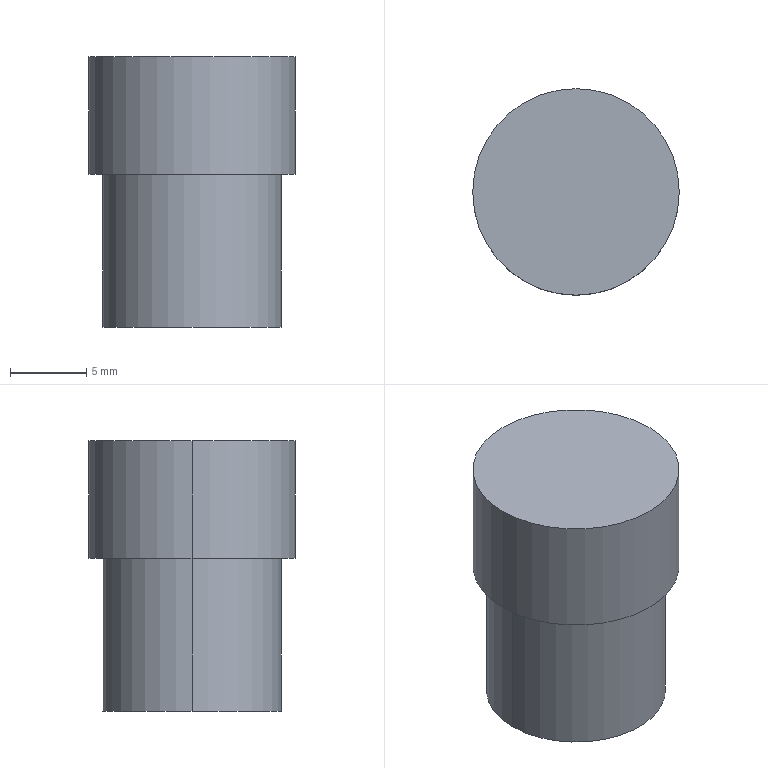Part | SolidWorks | features ICE 2, Extrusion 1 | 1 solid | 7 faces | box 13.5 x 13.5 x 17.7 mm | volume 2177 mm3 | cylinder 4 | plane 3 | commonest cylinder face diameters 11.7 x2 13.5 x2
STEP:
#1=CARTESIAN_POINT('',(44.682,-8.106,-13.2));
#2=VERTEX_POINT('',#1);
#3=CARTESIAN_POINT('',(56.382,-8.106,-13.2));
#4=VERTEX_POINT('',#3);
#5=CARTESIAN_POINT('',(50.532,-8.106,-13.2));
#6=DIRECTION('',(0.,0.,-1.));
#7=DIRECTION('',(-1.,0.,0.));
#8=AXIS2_PLACEMENT_3D('',#5,#6,#7);
#9=CIRCLE('',#8,5.85);
#10=EDGE_CURVE('',#2,#4,#9,.T.);
#11=ORIENTED_EDGE('',*,*,#10,.F.);
#12=CARTESIAN_POINT('',(44.682,-8.106,-3.2));
#13=VERTEX_POINT('',#12);
#14=CARTESIAN_POINT('',(44.682,-8.106,-13.2));
#15=DIRECTION('',(0.,0.,1.));
#16=VECTOR('',#15,1000.);
#17=LINE('',#14,#16);
#18=EDGE_CURVE('',#2,#13,#17,.T.);
#19=ORIENTED_EDGE('',*,*,#18,.T.);
#20=CARTESIAN_POINT('',(56.382,-8.106,-3.2));
#21=VERTEX_POINT('',#20);
#22=CARTESIAN_POINT('',(50.532,-8.106,-3.2));
#23=DIRECTION('',(0.,0.,-1.));
#24=DIRECTION('',(-1.,0.,0.));
#25=AXIS2_PLACEMENT_3D('',#22,#23,#24);
#26=CIRCLE('',#25,5.85);
#27=EDGE_CURVE('',#13,#21,#26,.T.);
#28=ORIENTED_EDGE('',*,*,#27,.T.);
#29=CARTESIAN_POINT('',(56.382,-8.106,-13.2));
#30=DIRECTION('',(0.,0.,1.));
#31=VECTOR('',#30,1000.);
#32=LINE('',#29,#31);
#33=EDGE_CURVE('',#4,#21,#32,.T.);
#34=ORIENTED_EDGE('',*,*,#33,.F.);
#35=EDGE_LOOP('',(#11,#19,#28,#34));
#36=FACE_OUTER_BOUND('',#35,.T.);
#37=CARTESIAN_POINT('',(50.532,-8.106,-13.2));
#38=DIRECTION('',(0.,0.,1.));
#39=DIRECTION('',(1.,0.,0.));
#40=AXIS2_PLACEMENT_3D('',#37,#38,#39);
#41=CYLINDRICAL_SURFACE('',#40,5.85);
#42=ADVANCED_FACE('',(#36),#41,.T.);
#43=CARTESIAN_POINT('',(57.282,-8.106,4.5));
#44=VERTEX_POINT('',#43);
#45=CARTESIAN_POINT('',(43.782,-8.106,4.5));
#46=VERTEX_POINT('',#45);
#47=CARTESIAN_POINT('',(50.532,-8.106,4.5));
#48=DIRECTION('',(0.,0.,1.));
#49=DIRECTION('',(1.,0.,0.));
#50=AXIS2_PLACEMENT_3D('',#47,#48,#49);
#51=CIRCLE('',#50,6.75);
#52=EDGE_CURVE('',#44,#46,#51,.T.);
#53=ORIENTED_EDGE('',*,*,#52,.F.);
#54=CARTESIAN_POINT('',(57.282,-8.106,-3.2));
#55=VERTEX_POINT('',#54);
#56=CARTESIAN_POINT('',(57.282,-8.106,4.5));
#57=DIRECTION('',(0.,0.,-1.));
#58=VECTOR('',#57,1000.);
#59=LINE('',#56,#58);
#60=EDGE_CURVE('',#44,#55,#59,.T.);
#61=ORIENTED_EDGE('',*,*,#60,.T.);
#62=CARTESIAN_POINT('',(43.782,-8.106,-3.2));
#63=VERTEX_POINT('',#62);
#64=CARTESIAN_POINT('',(50.532,-8.106,-3.2));
#65=DIRECTION('',(0.,0.,-1.));
#66=DIRECTION('',(-1.,0.,0.));
#67=AXIS2_PLACEMENT_3D('',#64,#65,#66);
#68=CIRCLE('',#67,6.75);
#69=EDGE_CURVE('',#63,#55,#68,.T.);
#70=ORIENTED_EDGE('',*,*,#69,.F.);
#71=CARTESIAN_POINT('',(43.782,-8.106,4.5));
#72=DIRECTION('',(0.,0.,-1.));
#73=VECTOR('',#72,1000.);
#74=LINE('',#71,#73);
#75=EDGE_CURVE('',#46,#63,#74,.T.);
#76=ORIENTED_EDGE('',*,*,#75,.F.);
#77=EDGE_LOOP('',(#53,#61,#70,#76));
#78=FACE_OUTER_BOUND('',#77,.T.);
#79=CARTESIAN_POINT('',(50.532,-8.106,4.5));
#80=DIRECTION('',(0.,0.,-1.));
#81=DIRECTION('',(-1.,0.,0.));
#82=AXIS2_PLACEMENT_3D('',#79,#80,#81);
#83=CYLINDRICAL_SURFACE('',#82,6.75);
#84=ADVANCED_FACE('',(#78),#83,.T.);
#85=ORIENTED_EDGE('',*,*,#60,.F.);
#86=CARTESIAN_POINT('',(50.532,-8.106,4.5));
#87=DIRECTION('',(0.,0.,1.));
#88=DIRECTION('',(1.,0.,0.));
#89=AXIS2_PLACEMENT_3D('',#86,#87,#88);
#90=CIRCLE('',#89,6.75);
#91=EDGE_CURVE('',#46,#44,#90,.T.);
#92=ORIENTED_EDGE('',*,*,#91,.F.);
#93=ORIENTED_EDGE('',*,*,#75,.T.);
#94=CARTESIAN_POINT('',(50.532,-8.106,-3.2));
#95=DIRECTION('',(0.,0.,-1.));
#96=DIRECTION('',(-1.,0.,0.));
#97=AXIS2_PLACEMENT_3D('',#94,#95,#96);
#98=CIRCLE('',#97,6.75);
#99=EDGE_CURVE('',#55,#63,#98,.T.);
#100=ORIENTED_EDGE('',*,*,#99,.F.);
#101=EDGE_LOOP('',(#85,#92,#93,#100));
#102=FACE_OUTER_BOUND('',#101,.T.);
#103=CARTESIAN_POINT('',(50.532,-8.106,4.5));
#104=DIRECTION('',(0.,0.,-1.));
#105=DIRECTION('',(-1.,0.,0.));
#106=AXIS2_PLACEMENT_3D('',#103,#104,#105);
#107=CYLINDRICAL_SURFACE('',#106,6.75);
#108=ADVANCED_FACE('',(#102),#107,.T.);
#109=ORIENTED_EDGE('',*,*,#91,.T.);
#110=ORIENTED_EDGE('',*,*,#52,.T.);
#111=EDGE_LOOP('',(#109,#110));
#112=FACE_OUTER_BOUND('',#111,.T.);
#113=CARTESIAN_POINT('',(50.532,-8.106,4.5));
#114=DIRECTION('',(0.,0.,1.));
#115=DIRECTION('',(1.,0.,0.));
#116=AXIS2_PLACEMENT_3D('',#113,#114,#115);
#117=PLANE('',#116);
#118=ADVANCED_FACE('',(#112),#117,.T.);
#119=CARTESIAN_POINT('',(50.532,-8.106,-3.2));
#120=DIRECTION('',(0.,0.,-1.));
#121=DIRECTION('',(-1.,0.,0.));
#122=AXIS2_PLACEMENT_3D('',#119,#120,#121);
#123=CIRCLE('',#122,5.85);
#124=EDGE_CURVE('',#21,#13,#123,.T.);
#125=ORIENTED_EDGE('',*,*,#124,.F.);
#126=ORIENTED_EDGE('',*,*,#27,.F.);
#127=EDGE_LOOP('',(#125,#126));
#128=FACE_BOUND('',#127,.T.);
#129=ORIENTED_EDGE('',*,*,#69,.T.);
#130=ORIENTED_EDGE('',*,*,#99,.T.);
#131=EDGE_LOOP('',(#129,#130));
#132=FACE_OUTER_BOUND('',#131,.T.);
#133=CARTESIAN_POINT('',(50.532,-8.106,-3.2));
#134=DIRECTION('',(0.,0.,-1.));
#135=DIRECTION('',(-1.,0.,0.));
#136=AXIS2_PLACEMENT_3D('',#133,#134,#135);
#137=PLANE('',#136);
#138=ADVANCED_FACE('',(#128,#132),#137,.T.);
#139=ORIENTED_EDGE('',*,*,#18,.F.);
#140=CARTESIAN_POINT('',(50.532,-8.106,-13.2));
#141=DIRECTION('',(0.,0.,-1.));
#142=DIRECTION('',(-1.,0.,0.));
#143=AXIS2_PLACEMENT_3D('',#140,#141,#142);
#144=CIRCLE('',#143,5.85);
#145=EDGE_CURVE('',#4,#2,#144,.T.);
#146=ORIENTED_EDGE('',*,*,#145,.F.);
#147=ORIENTED_EDGE('',*,*,#33,.T.);
#148=ORIENTED_EDGE('',*,*,#124,.T.);
#149=EDGE_LOOP('',(#139,#146,#147,#148));
#150=FACE_OUTER_BOUND('',#149,.T.);
#151=CARTESIAN_POINT('',(50.532,-8.106,-13.2));
#152=DIRECTION('',(0.,0.,1.));
#153=DIRECTION('',(1.,0.,0.));
#154=AXIS2_PLACEMENT_3D('',#151,#152,#153);
#155=CYLINDRICAL_SURFACE('',#154,5.85);
#156=ADVANCED_FACE('',(#150),#155,.T.);
#157=ORIENTED_EDGE('',*,*,#145,.T.);
#158=ORIENTED_EDGE('',*,*,#10,.T.);
#159=EDGE_LOOP('',(#157,#158));
#160=FACE_OUTER_BOUND('',#159,.T.);
#161=CARTESIAN_POINT('',(50.532,-8.106,-13.2));
#162=DIRECTION('',(0.,0.,-1.));
#163=DIRECTION('',(-1.,0.,0.));
#164=AXIS2_PLACEMENT_3D('',#161,#162,#163);
#165=PLANE('',#164);
#166=ADVANCED_FACE('',(#160),#165,.T.);
#167=CLOSED_SHELL('',(#42,#84,#108,#118,#138,#156,#166));
#168=MANIFOLD_SOLID_BREP('',#167);
#169=CARTESIAN_POINT('',(0.,0.,0.));
#170=DIRECTION('',(0.,0.,1.));
#171=DIRECTION('',(1.,0.,0.));
#172=AXIS2_PLACEMENT_3D('',#169,#170,#171);
#173=(LENGTH_UNIT()NAMED_UNIT(*)SI_UNIT(.MILLI.,.METRE.));
#174=UNCERTAINTY_MEASURE_WITH_UNIT(LENGTH_MEASURE(0.00001),#173,'','');
#175=(NAMED_UNIT(*)PLANE_ANGLE_UNIT()SI_UNIT($,.RADIAN.));
#176=(NAMED_UNIT(*)SI_UNIT($,.STERADIAN.)SOLID_ANGLE_UNIT());
#177=(GEOMETRIC_REPRESENTATION_CONTEXT(3)GLOBAL_UNCERTAINTY_ASSIGNED_CONTEXT((#174))GLOBAL_UNIT_ASSIGNED_CONTEXT((#173,#175,#176))REPRESENTATION_CONTEXT('',''));
#178=ADVANCED_BREP_SHAPE_REPRESENTATION('',(#168,#172),#177);